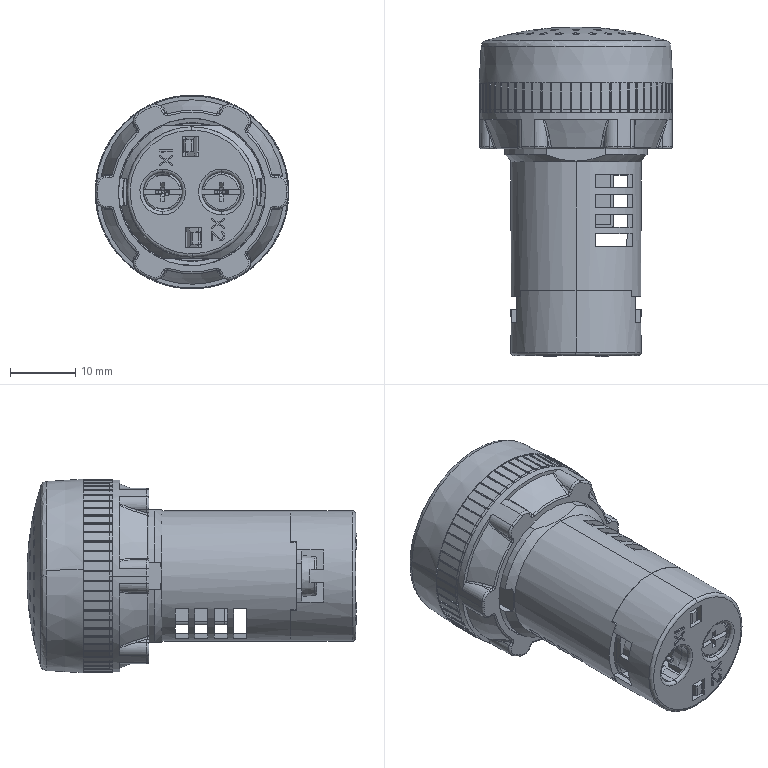Part | STEP file | Buzzer XB2BSB4LC | 18 solids | 1757 faces | box 29.699 x 50.596 x 29.699 mm | volume 12548 mm3 | plane 1010 | cylinder 501 | cone 91 | torus 83 | spline 64 | sphere 8 | commonest cylinder face diameters 1.199 x86 0.2 x76 29.699 x60 0.6 x44 1 x40 2.5 x16